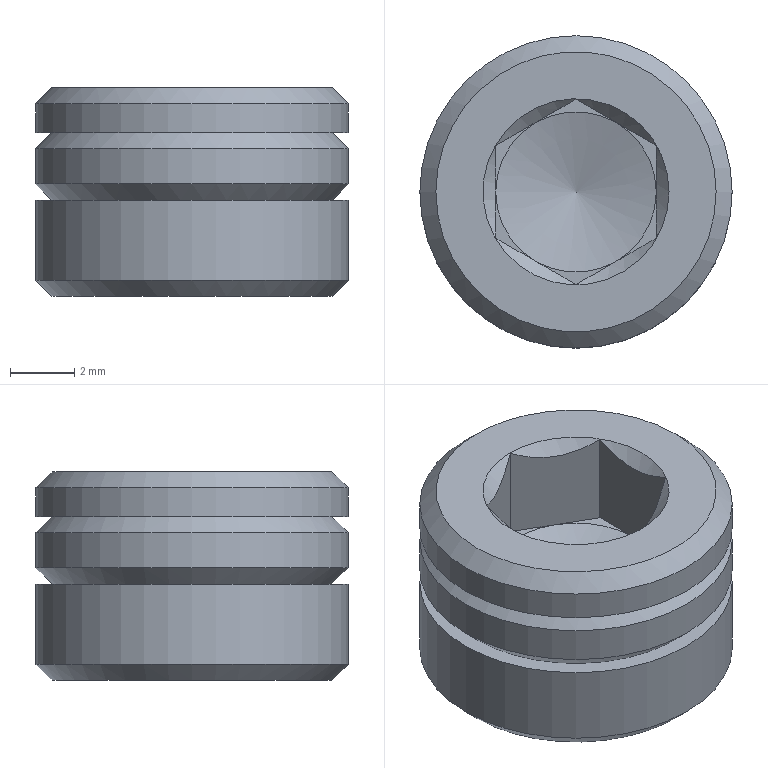Part | NX | features BREP 1 | 1 solid | 25 faces | box 9.728 x 9.728 x 6.5 mm | volume 398.103 mm3 | plane 16 | cone 6 | cylinder 3 | commonest cylinder face diameters 9.728 x3
STEP:
#1=CARTESIAN_POINT('',(4.364,0.,-6.5));
#2=VERTEX_POINT('',#1);
#3=CARTESIAN_POINT('',(0.,0.,-6.5));
#4=DIRECTION('',(0.,0.,1.));
#5=DIRECTION('',(1.,0.,0.));
#6=AXIS2_PLACEMENT_3D('',#3,#4,#5);
#7=CIRCLE('',#6,4.364);
#8=EDGE_CURVE('',#2,#2,#7,.T.);
#9=ORIENTED_EDGE('',*,*,#8,.F.);
#10=EDGE_LOOP('',(#9));
#11=FACE_BOUND('',#10,.T.);
#12=CARTESIAN_POINT('',(0.,4.364,-6.5));
#13=DIRECTION('',(0.,0.,1.));
#14=DIRECTION('',(-1.,0.,0.));
#15=AXIS2_PLACEMENT_3D('',#12,#13,#14);
#16=PLANE('',#15);
#17=ADVANCED_FACE('',(#11),#16,.F.);
#18=CARTESIAN_POINT('',(4.864,0.,-6.));
#19=VERTEX_POINT('',#18);
#20=CARTESIAN_POINT('',(0.,0.,-6.));
#21=DIRECTION('',(0.,0.,-1.));
#22=DIRECTION('',(1.,0.,0.));
#23=AXIS2_PLACEMENT_3D('',#20,#21,#22);
#24=CIRCLE('',#23,4.864);
#25=EDGE_CURVE('',#19,#19,#24,.T.);
#26=ORIENTED_EDGE('',*,*,#25,.T.);
#27=EDGE_LOOP('',(#26));
#28=FACE_BOUND('',#27,.T.);
#29=ORIENTED_EDGE('',*,*,#8,.T.);
#30=EDGE_LOOP('',(#29));
#31=FACE_BOUND('',#30,.T.);
#32=CARTESIAN_POINT('',(0.,0.,-6.));
#33=DIRECTION('',(0.,0.,1.));
#34=DIRECTION('',(-1.,0.,0.));
#35=AXIS2_PLACEMENT_3D('',#32,#33,#34);
#36=CONICAL_SURFACE('',#35,4.864,0.7854);
#37=ADVANCED_FACE('',(#28,#31),#36,.T.);
#38=CARTESIAN_POINT('',(4.864,0.,-3.5));
#39=VERTEX_POINT('',#38);
#40=CARTESIAN_POINT('',(0.,0.,-3.5));
#41=DIRECTION('',(0.,0.,-1.));
#42=DIRECTION('',(1.,0.,0.));
#43=AXIS2_PLACEMENT_3D('',#40,#41,#42);
#44=CIRCLE('',#43,4.864);
#45=EDGE_CURVE('',#39,#39,#44,.T.);
#46=ORIENTED_EDGE('',*,*,#45,.T.);
#47=EDGE_LOOP('',(#46));
#48=FACE_BOUND('',#47,.T.);
#49=ORIENTED_EDGE('',*,*,#25,.F.);
#50=EDGE_LOOP('',(#49));
#51=FACE_BOUND('',#50,.T.);
#52=CARTESIAN_POINT('',(0.,0.,-6.5));
#53=DIRECTION('',(0.,0.,1.));
#54=DIRECTION('',(-1.,0.,0.));
#55=AXIS2_PLACEMENT_3D('',#52,#53,#54);
#56=CYLINDRICAL_SURFACE('',#55,4.864);
#57=ADVANCED_FACE('',(#48,#51),#56,.T.);
#58=CARTESIAN_POINT('',(4.364,0.,-3.5));
#59=VERTEX_POINT('',#58);
#60=CARTESIAN_POINT('',(0.,0.,-3.5));
#61=DIRECTION('',(0.,0.,-1.));
#62=DIRECTION('',(1.,0.,0.));
#63=AXIS2_PLACEMENT_3D('',#60,#61,#62);
#64=CIRCLE('',#63,4.364);
#65=EDGE_CURVE('',#59,#59,#64,.T.);
#66=ORIENTED_EDGE('',*,*,#65,.T.);
#67=EDGE_LOOP('',(#66));
#68=FACE_BOUND('',#67,.T.);
#69=ORIENTED_EDGE('',*,*,#45,.F.);
#70=EDGE_LOOP('',(#69));
#71=FACE_BOUND('',#70,.T.);
#72=CARTESIAN_POINT('',(0.,4.364,-3.5));
#73=DIRECTION('',(0.,0.,1.));
#74=DIRECTION('',(-1.,0.,0.));
#75=AXIS2_PLACEMENT_3D('',#72,#73,#74);
#76=PLANE('',#75);
#77=ADVANCED_FACE('',(#68,#71),#76,.T.);
#78=ORIENTED_EDGE('',*,*,#65,.F.);
#79=EDGE_LOOP('',(#78));
#80=FACE_BOUND('',#79,.T.);
#81=CARTESIAN_POINT('',(4.864,0.,-3.));
#82=VERTEX_POINT('',#81);
#83=CARTESIAN_POINT('',(0.,0.,-3.));
#84=DIRECTION('',(0.,0.,-1.));
#85=DIRECTION('',(1.,0.,0.));
#86=AXIS2_PLACEMENT_3D('',#83,#84,#85);
#87=CIRCLE('',#86,4.864);
#88=EDGE_CURVE('',#82,#82,#87,.T.);
#89=ORIENTED_EDGE('',*,*,#88,.T.);
#90=EDGE_LOOP('',(#89));
#91=FACE_BOUND('',#90,.T.);
#92=CARTESIAN_POINT('',(0.,0.,-3.));
#93=DIRECTION('',(0.,0.,1.));
#94=DIRECTION('',(-1.,0.,0.));
#95=AXIS2_PLACEMENT_3D('',#92,#93,#94);
#96=CONICAL_SURFACE('',#95,4.864,0.7854);
#97=ADVANCED_FACE('',(#80,#91),#96,.T.);
#98=ORIENTED_EDGE('',*,*,#88,.F.);
#99=EDGE_LOOP('',(#98));
#100=FACE_BOUND('',#99,.T.);
#101=CARTESIAN_POINT('',(4.864,0.,-1.9));
#102=VERTEX_POINT('',#101);
#103=CARTESIAN_POINT('',(0.,0.,-1.9));
#104=DIRECTION('',(0.,0.,-1.));
#105=DIRECTION('',(1.,0.,0.));
#106=AXIS2_PLACEMENT_3D('',#103,#104,#105);
#107=CIRCLE('',#106,4.864);
#108=EDGE_CURVE('',#102,#102,#107,.T.);
#109=ORIENTED_EDGE('',*,*,#108,.T.);
#110=EDGE_LOOP('',(#109));
#111=FACE_BOUND('',#110,.T.);
#112=CARTESIAN_POINT('',(0.,0.,-6.5));
#113=DIRECTION('',(0.,0.,1.));
#114=DIRECTION('',(-1.,0.,0.));
#115=AXIS2_PLACEMENT_3D('',#112,#113,#114);
#116=CYLINDRICAL_SURFACE('',#115,4.864);
#117=ADVANCED_FACE('',(#100,#111),#116,.T.);
#118=CARTESIAN_POINT('',(-4.364,0.,-1.4));
#119=VERTEX_POINT('',#118);
#120=CARTESIAN_POINT('',(0.,0.,-1.4));
#121=DIRECTION('',(0.,0.,-1.));
#122=DIRECTION('',(-1.,0.,0.));
#123=AXIS2_PLACEMENT_3D('',#120,#121,#122);
#124=CIRCLE('',#123,4.364);
#125=EDGE_CURVE('',#119,#119,#124,.T.);
#126=ORIENTED_EDGE('',*,*,#125,.T.);
#127=EDGE_LOOP('',(#126));
#128=FACE_BOUND('',#127,.T.);
#129=ORIENTED_EDGE('',*,*,#108,.F.);
#130=EDGE_LOOP('',(#129));
#131=FACE_BOUND('',#130,.T.);
#132=CARTESIAN_POINT('',(0.,0.,-1.9));
#133=DIRECTION('',(0.,0.,-1.));
#134=DIRECTION('',(1.,0.,0.));
#135=AXIS2_PLACEMENT_3D('',#132,#133,#134);
#136=CONICAL_SURFACE('',#135,4.864,0.7854);
#137=ADVANCED_FACE('',(#128,#131),#136,.T.);
#138=CARTESIAN_POINT('',(4.864,0.,-1.4));
#139=VERTEX_POINT('',#138);
#140=CARTESIAN_POINT('',(0.,0.,-1.4));
#141=DIRECTION('',(0.,0.,-1.));
#142=DIRECTION('',(1.,0.,0.));
#143=AXIS2_PLACEMENT_3D('',#140,#141,#142);
#144=CIRCLE('',#143,4.864);
#145=EDGE_CURVE('',#139,#139,#144,.T.);
#146=ORIENTED_EDGE('',*,*,#145,.T.);
#147=EDGE_LOOP('',(#146));
#148=FACE_BOUND('',#147,.T.);
#149=ORIENTED_EDGE('',*,*,#125,.F.);
#150=EDGE_LOOP('',(#149));
#151=FACE_BOUND('',#150,.T.);
#152=CARTESIAN_POINT('',(0.,4.864,-1.4));
#153=DIRECTION('',(0.,0.,-1.));
#154=DIRECTION('',(1.,0.,0.));
#155=AXIS2_PLACEMENT_3D('',#152,#153,#154);
#156=PLANE('',#155);
#157=ADVANCED_FACE('',(#148,#151),#156,.T.);
#158=ORIENTED_EDGE('',*,*,#145,.F.);
#159=EDGE_LOOP('',(#158));
#160=FACE_BOUND('',#159,.T.);
#161=CARTESIAN_POINT('',(4.864,0.,-0.5));
#162=VERTEX_POINT('',#161);
#163=CARTESIAN_POINT('',(0.,0.,-0.5));
#164=DIRECTION('',(0.,0.,-1.));
#165=DIRECTION('',(1.,0.,0.));
#166=AXIS2_PLACEMENT_3D('',#163,#164,#165);
#167=CIRCLE('',#166,4.864);
#168=EDGE_CURVE('',#162,#162,#167,.T.);
#169=ORIENTED_EDGE('',*,*,#168,.T.);
#170=EDGE_LOOP('',(#169));
#171=FACE_BOUND('',#170,.T.);
#172=CARTESIAN_POINT('',(0.,0.,-6.5));
#173=DIRECTION('',(0.,0.,1.));
#174=DIRECTION('',(-1.,0.,0.));
#175=AXIS2_PLACEMENT_3D('',#172,#173,#174);
#176=CYLINDRICAL_SURFACE('',#175,4.864);
#177=ADVANCED_FACE('',(#160,#171),#176,.T.);
#178=CARTESIAN_POINT('',(-4.364,0.,0.));
#179=VERTEX_POINT('',#178);
#180=CARTESIAN_POINT('',(0.,0.,0.));
#181=DIRECTION('',(0.,0.,-1.));
#182=DIRECTION('',(-1.,0.,0.));
#183=AXIS2_PLACEMENT_3D('',#180,#181,#182);
#184=CIRCLE('',#183,4.364);
#185=EDGE_CURVE('',#179,#179,#184,.T.);
#186=ORIENTED_EDGE('',*,*,#185,.T.);
#187=EDGE_LOOP('',(#186));
#188=FACE_BOUND('',#187,.T.);
#189=ORIENTED_EDGE('',*,*,#168,.F.);
#190=EDGE_LOOP('',(#189));
#191=FACE_BOUND('',#190,.T.);
#192=CARTESIAN_POINT('',(0.,0.,-0.5));
#193=DIRECTION('',(0.,0.,-1.));
#194=DIRECTION('',(1.,0.,0.));
#195=AXIS2_PLACEMENT_3D('',#192,#193,#194);
#196=CONICAL_SURFACE('',#195,4.864,0.7854);
#197=ADVANCED_FACE('',(#188,#191),#196,.T.);
#198=ORIENTED_EDGE('',*,*,#185,.F.);
#199=EDGE_LOOP('',(#198));
#200=FACE_BOUND('',#199,.T.);
#201=CARTESIAN_POINT('',(2.9,0.,0.));
#202=VERTEX_POINT('',#201);
#203=CARTESIAN_POINT('',(0.,0.,0.));
#204=DIRECTION('',(0.,0.,1.));
#205=DIRECTION('',(1.,0.,0.));
#206=AXIS2_PLACEMENT_3D('',#203,#204,#205);
#207=CIRCLE('',#206,2.9);
#208=EDGE_CURVE('',#202,#202,#207,.T.);
#209=ORIENTED_EDGE('',*,*,#208,.F.);
#210=EDGE_LOOP('',(#209));
#211=FACE_BOUND('',#210,.T.);
#212=CARTESIAN_POINT('',(0.,0.,0.));
#213=DIRECTION('',(0.,0.,-1.));
#214=DIRECTION('',(1.,0.,0.));
#215=AXIS2_PLACEMENT_3D('',#212,#213,#214);
#216=PLANE('',#215);
#217=ADVANCED_FACE('',(#200,#211),#216,.F.);
#218=CARTESIAN_POINT('',(2.5,1.443,-0.01325));
#219=VERTEX_POINT('',#218);
#220=CARTESIAN_POINT('',(2.5,-1.443,-0.01325));
#221=VERTEX_POINT('',#220);
#222=CARTESIAN_POINT('',(2.5,1.443,-0.01325));
#223=CARTESIAN_POINT('',(2.5,0.9923,-0.2388));
#224=CARTESIAN_POINT('',(2.5,0.009298,-0.5605));
#225=CARTESIAN_POINT('',(2.5,-0.9896,-0.2401));
#226=CARTESIAN_POINT('',(2.5,-1.443,-0.01325));
#227=B_SPLINE_CURVE_WITH_KNOTS('',3,(#222,#223,#224,#225,#226),.UNSPECIFIED.,.F.,.F.,(4,1,4),(0.,0.001491,0.002982),.UNSPECIFIED.);
#228=EDGE_CURVE('',#219,#221,#227,.T.);
#229=ORIENTED_EDGE('',*,*,#228,.T.);
#230=CARTESIAN_POINT('',(-0.000000007,-2.887,-0.01325));
#231=VERTEX_POINT('',#230);
#232=CARTESIAN_POINT('',(-0.000000012,-2.887,-0.01325));
#233=CARTESIAN_POINT('',(0.3907,-2.661,-0.2388));
#234=CARTESIAN_POINT('',(1.242,-2.17,-0.5605));
#235=CARTESIAN_POINT('',(2.107,-1.67,-0.2401));
#236=CARTESIAN_POINT('',(2.5,-1.443,-0.01325));
#237=B_SPLINE_CURVE_WITH_KNOTS('',3,(#232,#233,#234,#235,#236),.UNSPECIFIED.,.F.,.F.,(4,1,4),(0.,0.001491,0.002982),.UNSPECIFIED.);
#238=EDGE_CURVE('',#231,#221,#237,.T.);
#239=ORIENTED_EDGE('',*,*,#238,.F.);
#240=CARTESIAN_POINT('',(-2.5,-1.443,-0.01325));
#241=VERTEX_POINT('',#240);
#242=CARTESIAN_POINT('',(-2.5,-1.443,-0.01325));
#243=CARTESIAN_POINT('',(-2.109,-1.669,-0.2388));
#244=CARTESIAN_POINT('',(-1.258,-2.16,-0.5605));
#245=CARTESIAN_POINT('',(-0.393,-2.66,-0.2401));
#246=CARTESIAN_POINT('',(-0.000000002,-2.887,-0.01325));
#247=B_SPLINE_CURVE_WITH_KNOTS('',3,(#242,#243,#244,#245,#246),.UNSPECIFIED.,.F.,.F.,(4,1,4),(0.,0.001491,0.002982),.UNSPECIFIED.);
#248=EDGE_CURVE('',#241,#231,#247,.T.);
#249=ORIENTED_EDGE('',*,*,#248,.F.);
#250=CARTESIAN_POINT('',(-2.5,1.443,-0.01325));
#251=VERTEX_POINT('',#250);
#252=CARTESIAN_POINT('',(-2.5,-1.443,-0.01325));
#253=CARTESIAN_POINT('',(-2.5,-0.9923,-0.2388));
#254=CARTESIAN_POINT('',(-2.5,-0.009298,-0.5605));
#255=CARTESIAN_POINT('',(-2.5,0.9896,-0.2401));
#256=CARTESIAN_POINT('',(-2.5,1.443,-0.01325));
#257=B_SPLINE_CURVE_WITH_KNOTS('',3,(#252,#253,#254,#255,#256),.UNSPECIFIED.,.F.,.F.,(4,1,4),(0.,0.001491,0.002982),.UNSPECIFIED.);
#258=EDGE_CURVE('',#241,#251,#257,.T.);
#259=ORIENTED_EDGE('',*,*,#258,.T.);
#260=CARTESIAN_POINT('',(0.000000007,2.887,-0.01325));
#261=VERTEX_POINT('',#260);
#262=CARTESIAN_POINT('',(0.000000012,2.887,-0.01325));
#263=CARTESIAN_POINT('',(-0.3907,2.661,-0.2388));
#264=CARTESIAN_POINT('',(-1.242,2.17,-0.5605));
#265=CARTESIAN_POINT('',(-2.107,1.67,-0.2401));
#266=CARTESIAN_POINT('',(-2.5,1.443,-0.01325));
#267=B_SPLINE_CURVE_WITH_KNOTS('',3,(#262,#263,#264,#265,#266),.UNSPECIFIED.,.F.,.F.,(4,1,4),(0.,0.001491,0.002982),.UNSPECIFIED.);
#268=EDGE_CURVE('',#261,#251,#267,.T.);
#269=ORIENTED_EDGE('',*,*,#268,.F.);
#270=CARTESIAN_POINT('',(2.5,1.443,-0.01325));
#271=CARTESIAN_POINT('',(2.109,1.669,-0.2388));
#272=CARTESIAN_POINT('',(1.258,2.16,-0.5605));
#273=CARTESIAN_POINT('',(0.393,2.66,-0.2401));
#274=CARTESIAN_POINT('',(0.000000002,2.887,-0.01325));
#275=B_SPLINE_CURVE_WITH_KNOTS('',3,(#270,#271,#272,#273,#274),.UNSPECIFIED.,.F.,.F.,(4,1,4),(0.,0.001491,0.002982),.UNSPECIFIED.);
#276=EDGE_CURVE('',#219,#261,#275,.T.);
#277=ORIENTED_EDGE('',*,*,#276,.F.);
#278=EDGE_LOOP('',(#229,#239,#249,#259,#269,#277));
#279=FACE_BOUND('',#278,.T.);
#280=ORIENTED_EDGE('',*,*,#208,.T.);
#281=EDGE_LOOP('',(#280));
#282=FACE_BOUND('',#281,.T.);
#283=CARTESIAN_POINT('',(0.,0.,0.));
#284=DIRECTION('',(0.,0.,1.));
#285=DIRECTION('',(-1.,0.,0.));
#286=AXIS2_PLACEMENT_3D('',#283,#284,#285);
#287=CONICAL_SURFACE('',#286,2.9,0.7854);
#288=ADVANCED_FACE('',(#279,#282),#287,.F.);
#289=CARTESIAN_POINT('',(-2.5,1.443,-3.));
#290=VERTEX_POINT('',#289);
#291=CARTESIAN_POINT('',(-2.5,1.443,-3.));
#292=DIRECTION('',(0.,0.,1.));
#293=VECTOR('',#292,1000.);
#294=LINE('',#291,#293);
#295=EDGE_CURVE('',#290,#251,#294,.T.);
#296=ORIENTED_EDGE('',*,*,#295,.F.);
#297=CARTESIAN_POINT('',(-1.25,2.165,-3.));
#298=VERTEX_POINT('',#297);
#299=CARTESIAN_POINT('',(-1.25,2.165,-3.));
#300=DIRECTION('',(-0.866,-0.5,0.));
#301=VECTOR('',#300,1000.);
#302=LINE('',#299,#301);
#303=EDGE_CURVE('',#298,#290,#302,.T.);
#304=ORIENTED_EDGE('',*,*,#303,.F.);
#305=CARTESIAN_POINT('',(0.,2.887,-3.));
#306=VERTEX_POINT('',#305);
#307=CARTESIAN_POINT('',(0.,2.887,-3.));
#308=DIRECTION('',(-0.866,-0.5,0.));
#309=VECTOR('',#308,1000.);
#310=LINE('',#307,#309);
#311=EDGE_CURVE('',#306,#298,#310,.T.);
#312=ORIENTED_EDGE('',*,*,#311,.F.);
#313=CARTESIAN_POINT('',(0.,2.887,-3.));
#314=DIRECTION('',(0.,0.,-1.));
#315=VECTOR('',#314,1000.);
#316=LINE('',#313,#315);
#317=EDGE_CURVE('',#261,#306,#316,.T.);
#318=ORIENTED_EDGE('',*,*,#317,.F.);
#319=ORIENTED_EDGE('',*,*,#268,.T.);
#320=EDGE_LOOP('',(#296,#304,#312,#318,#319));
#321=FACE_BOUND('',#320,.T.);
#322=CARTESIAN_POINT('',(0.,2.887,-3.));
#323=DIRECTION('',(-0.5,0.866,0.));
#324=DIRECTION('',(0.866,0.5,0.));
#325=AXIS2_PLACEMENT_3D('',#322,#323,#324);
#326=PLANE('',#325);
#327=ADVANCED_FACE('',(#321),#326,.F.);
#328=ORIENTED_EDGE('',*,*,#317,.T.);
#329=CARTESIAN_POINT('',(1.25,2.165,-3.));
#330=VERTEX_POINT('',#329);
#331=CARTESIAN_POINT('',(1.25,2.165,-3.));
#332=DIRECTION('',(-0.866,0.5,0.));
#333=VECTOR('',#332,1000.);
#334=LINE('',#331,#333);
#335=EDGE_CURVE('',#330,#306,#334,.T.);
#336=ORIENTED_EDGE('',*,*,#335,.F.);
#337=CARTESIAN_POINT('',(2.5,1.443,-3.));
#338=VERTEX_POINT('',#337);
#339=CARTESIAN_POINT('',(2.5,1.443,-3.));
#340=DIRECTION('',(-0.866,0.5,0.));
#341=VECTOR('',#340,1000.);
#342=LINE('',#339,#341);
#343=EDGE_CURVE('',#338,#330,#342,.T.);
#344=ORIENTED_EDGE('',*,*,#343,.F.);
#345=CARTESIAN_POINT('',(2.5,1.443,-3.));
#346=DIRECTION('',(0.,0.,-1.));
#347=VECTOR('',#346,1000.);
#348=LINE('',#345,#347);
#349=EDGE_CURVE('',#219,#338,#348,.T.);
#350=ORIENTED_EDGE('',*,*,#349,.F.);
#351=ORIENTED_EDGE('',*,*,#276,.T.);
#352=EDGE_LOOP('',(#328,#336,#344,#350,#351));
#353=FACE_BOUND('',#352,.T.);
#354=CARTESIAN_POINT('',(2.5,1.443,-3.));
#355=DIRECTION('',(0.5,0.866,0.));
#356=DIRECTION('',(0.866,-0.5,0.));
#357=AXIS2_PLACEMENT_3D('',#354,#355,#356);
#358=PLANE('',#357);
#359=ADVANCED_FACE('',(#353),#358,.F.);
#360=CARTESIAN_POINT('',(2.5,-1.443,-3.));
#361=VERTEX_POINT('',#360);
#362=CARTESIAN_POINT('',(2.5,-1.443,-3.));
#363=DIRECTION('',(0.,0.,1.));
#364=VECTOR('',#363,1000.);
#365=LINE('',#362,#364);
#366=EDGE_CURVE('',#361,#221,#365,.T.);
#367=ORIENTED_EDGE('',*,*,#366,.F.);
#368=CARTESIAN_POINT('',(1.25,-2.165,-3.));
#369=VERTEX_POINT('',#368);
#370=CARTESIAN_POINT('',(1.25,-2.165,-3.));
#371=DIRECTION('',(0.866,0.5,0.));
#372=VECTOR('',#371,1000.);
#373=LINE('',#370,#372);
#374=EDGE_CURVE('',#369,#361,#373,.T.);
#375=ORIENTED_EDGE('',*,*,#374,.F.);
#376=CARTESIAN_POINT('',(0.,-2.887,-3.));
#377=VERTEX_POINT('',#376);
#378=CARTESIAN_POINT('',(0.,-2.887,-3.));
#379=DIRECTION('',(0.866,0.5,0.));
#380=VECTOR('',#379,1000.);
#381=LINE('',#378,#380);
#382=EDGE_CURVE('',#377,#369,#381,.T.);
#383=ORIENTED_EDGE('',*,*,#382,.F.);
#384=CARTESIAN_POINT('',(0.,-2.887,-3.));
#385=DIRECTION('',(0.,0.,-1.));
#386=VECTOR('',#385,1000.);
#387=LINE('',#384,#386);
#388=EDGE_CURVE('',#231,#377,#387,.T.);
#389=ORIENTED_EDGE('',*,*,#388,.F.);
#390=ORIENTED_EDGE('',*,*,#238,.T.);
#391=EDGE_LOOP('',(#367,#375,#383,#389,#390));
#392=FACE_BOUND('',#391,.T.);
#393=CARTESIAN_POINT('',(0.,-2.887,-3.));
#394=DIRECTION('',(0.5,-0.866,0.));
#395=DIRECTION('',(-0.866,-0.5,0.));
#396=AXIS2_PLACEMENT_3D('',#393,#394,#395);
#397=PLANE('',#396);
#398=ADVANCED_FACE('',(#392),#397,.F.);
#399=ORIENTED_EDGE('',*,*,#388,.T.);
#400=CARTESIAN_POINT('',(-1.25,-2.165,-3.));
#401=VERTEX_POINT('',#400);
#402=CARTESIAN_POINT('',(-1.25,-2.165,-3.));
#403=DIRECTION('',(0.866,-0.5,0.));
#404=VECTOR('',#403,1000.);
#405=LINE('',#402,#404);
#406=EDGE_CURVE('',#401,#377,#405,.T.);
#407=ORIENTED_EDGE('',*,*,#406,.F.);
#408=CARTESIAN_POINT('',(-2.5,-1.443,-3.));
#409=VERTEX_POINT('',#408);
#410=CARTESIAN_POINT('',(-2.5,-1.443,-3.));
#411=DIRECTION('',(0.866,-0.5,0.));
#412=VECTOR('',#411,1000.);
#413=LINE('',#410,#412);
#414=EDGE_CURVE('',#409,#401,#413,.T.);
#415=ORIENTED_EDGE('',*,*,#414,.F.);
#416=CARTESIAN_POINT('',(-2.5,-1.443,-3.));
#417=DIRECTION('',(0.,0.,-1.));
#418=VECTOR('',#417,1000.);
#419=LINE('',#416,#418);
#420=EDGE_CURVE('',#241,#409,#419,.T.);
#421=ORIENTED_EDGE('',*,*,#420,.F.);
#422=ORIENTED_EDGE('',*,*,#248,.T.);
#423=EDGE_LOOP('',(#399,#407,#415,#421,#422));
#424=FACE_BOUND('',#423,.T.);
#425=CARTESIAN_POINT('',(-2.5,-1.443,-3.));
#426=DIRECTION('',(-0.5,-0.866,0.));
#427=DIRECTION('',(-0.866,0.5,0.));
#428=AXIS2_PLACEMENT_3D('',#425,#426,#427);
#429=PLANE('',#428);
#430=ADVANCED_FACE('',(#424),#429,.F.);
#431=ORIENTED_EDGE('',*,*,#420,.T.);
#432=CARTESIAN_POINT('',(-2.5,0.,-3.));
#433=VERTEX_POINT('',#432);
#434=CARTESIAN_POINT('',(-2.5,1.443,-3.));
#435=DIRECTION('',(0.,-1.,0.));
#436=VECTOR('',#435,1000.);
#437=LINE('',#434,#436);
#438=EDGE_CURVE('',#433,#409,#437,.T.);
#439=ORIENTED_EDGE('',*,*,#438,.F.);
#440=CARTESIAN_POINT('',(-2.5,0.,-3.));
#441=DIRECTION('',(0.,-1.,0.));
#442=VECTOR('',#441,1000.);
#443=LINE('',#440,#442);
#444=EDGE_CURVE('',#290,#433,#443,.T.);
#445=ORIENTED_EDGE('',*,*,#444,.F.);
#446=ORIENTED_EDGE('',*,*,#295,.T.);
#447=ORIENTED_EDGE('',*,*,#258,.F.);
#448=EDGE_LOOP('',(#431,#439,#445,#446,#447));
#449=FACE_BOUND('',#448,.T.);
#450=CARTESIAN_POINT('',(-2.5,1.443,-3.));
#451=DIRECTION('',(-1.,0.,0.));
#452=DIRECTION('',(0.,0.,-1.));
#453=AXIS2_PLACEMENT_3D('',#450,#451,#452);
#454=PLANE('',#453);
#455=ADVANCED_FACE('',(#449),#454,.F.);
#456=ORIENTED_EDGE('',*,*,#349,.T.);
#457=CARTESIAN_POINT('',(2.5,0.,-3.));
#458=VERTEX_POINT('',#457);
#459=CARTESIAN_POINT('',(2.5,0.,-3.));
#460=DIRECTION('',(0.,1.,0.));
#461=VECTOR('',#460,1000.);
#462=LINE('',#459,#461);
#463=EDGE_CURVE('',#458,#338,#462,.T.);
#464=ORIENTED_EDGE('',*,*,#463,.F.);
#465=CARTESIAN_POINT('',(2.5,0.,-3.));
#466=DIRECTION('',(0.,1.,0.));
#467=VECTOR('',#466,1000.);
#468=LINE('',#465,#467);
#469=EDGE_CURVE('',#361,#458,#468,.T.);
#470=ORIENTED_EDGE('',*,*,#469,.F.);
#471=ORIENTED_EDGE('',*,*,#366,.T.);
#472=ORIENTED_EDGE('',*,*,#228,.F.);
#473=EDGE_LOOP('',(#456,#464,#470,#471,#472));
#474=FACE_BOUND('',#473,.T.);
#475=CARTESIAN_POINT('',(2.5,-1.443,-3.));
#476=DIRECTION('',(1.,0.,0.));
#477=DIRECTION('',(0.,0.,1.));
#478=AXIS2_PLACEMENT_3D('',#475,#476,#477);
#479=PLANE('',#478);
#480=ADVANCED_FACE('',(#474),#479,.F.);
#481=ORIENTED_EDGE('',*,*,#438,.T.);
#482=ORIENTED_EDGE('',*,*,#414,.T.);
#483=CARTESIAN_POINT('',(0.,0.,-3.));
#484=DIRECTION('',(0.,0.,-1.));
#485=DIRECTION('',(1.,0.,0.));
#486=AXIS2_PLACEMENT_3D('',#483,#484,#485);
#487=CIRCLE('',#486,2.5);
#488=EDGE_CURVE('',#401,#433,#487,.T.);
#489=ORIENTED_EDGE('',*,*,#488,.T.);
#490=EDGE_LOOP('',(#481,#482,#489));
#491=FACE_BOUND('',#490,.T.);
#492=CARTESIAN_POINT('',(0.,0.,-3.));
#493=DIRECTION('',(0.,0.,1.));
#494=DIRECTION('',(-1.,0.,0.));
#495=AXIS2_PLACEMENT_3D('',#492,#493,#494);
#496=PLANE('',#495);
#497=ADVANCED_FACE('',(#491),#496,.T.);
#498=CARTESIAN_POINT('',(0.,0.,-3.693));
#499=VERTEX_POINT('',#498);
#500=VERTEX_LOOP('',#499);
#501=FACE_BOUND('',#500,.T.);
#502=CARTESIAN_POINT('',(0.,0.,-3.));
#503=DIRECTION('',(0.,0.,-1.));
#504=DIRECTION('',(1.,0.,0.));
#505=AXIS2_PLACEMENT_3D('',#502,#503,#504);
#506=CIRCLE('',#505,2.5);
#507=EDGE_CURVE('',#433,#298,#506,.T.);
#508=ORIENTED_EDGE('',*,*,#507,.F.);
#509=ORIENTED_EDGE('',*,*,#488,.F.);
#510=CARTESIAN_POINT('',(0.,0.,-3.));
#511=DIRECTION('',(0.,0.,-1.));
#512=DIRECTION('',(1.,0.,0.));
#513=AXIS2_PLACEMENT_3D('',#510,#511,#512);
#514=CIRCLE('',#513,2.5);
#515=EDGE_CURVE('',#369,#401,#514,.T.);
#516=ORIENTED_EDGE('',*,*,#515,.F.);
#517=CARTESIAN_POINT('',(0.,0.,-3.));
#518=DIRECTION('',(0.,0.,-1.));
#519=DIRECTION('',(1.,0.,0.));
#520=AXIS2_PLACEMENT_3D('',#517,#518,#519);
#521=CIRCLE('',#520,2.5);
#522=EDGE_CURVE('',#458,#369,#521,.T.);
#523=ORIENTED_EDGE('',*,*,#522,.F.);
#524=CARTESIAN_POINT('',(0.,0.,-3.));
#525=DIRECTION('',(0.,0.,-1.));
#526=DIRECTION('',(1.,0.,0.));
#527=AXIS2_PLACEMENT_3D('',#524,#525,#526);
#528=CIRCLE('',#527,2.5);
#529=EDGE_CURVE('',#330,#458,#528,.T.);
#530=ORIENTED_EDGE('',*,*,#529,.F.);
#531=CARTESIAN_POINT('',(0.,0.,-3.));
#532=DIRECTION('',(0.,0.,-1.));
#533=DIRECTION('',(1.,0.,0.));
#534=AXIS2_PLACEMENT_3D('',#531,#532,#533);
#535=CIRCLE('',#534,2.5);
#536=EDGE_CURVE('',#298,#330,#535,.T.);
#537=ORIENTED_EDGE('',*,*,#536,.F.);
#538=EDGE_LOOP('',(#508,#509,#516,#523,#530,#537));
#539=FACE_BOUND('',#538,.T.);
#540=CARTESIAN_POINT('',(0.,0.,-3.));
#541=DIRECTION('',(0.,0.,1.));
#542=DIRECTION('',(-1.,0.,0.));
#543=AXIS2_PLACEMENT_3D('',#540,#541,#542);
#544=CONICAL_SURFACE('',#543,2.5,1.3);
#545=ADVANCED_FACE('',(#501,#539),#544,.F.);
#546=ORIENTED_EDGE('',*,*,#406,.T.);
#547=ORIENTED_EDGE('',*,*,#382,.T.);
#548=ORIENTED_EDGE('',*,*,#515,.T.);
#549=EDGE_LOOP('',(#546,#547,#548));
#550=FACE_BOUND('',#549,.T.);
#551=CARTESIAN_POINT('',(0.,0.,-3.));
#552=DIRECTION('',(0.,0.,1.));
#553=DIRECTION('',(-1.,0.,0.));
#554=AXIS2_PLACEMENT_3D('',#551,#552,#553);
#555=PLANE('',#554);
#556=ADVANCED_FACE('',(#550),#555,.T.);
#557=ORIENTED_EDGE('',*,*,#374,.T.);
#558=ORIENTED_EDGE('',*,*,#469,.T.);
#559=ORIENTED_EDGE('',*,*,#522,.T.);
#560=EDGE_LOOP('',(#557,#558,#559));
#561=FACE_BOUND('',#560,.T.);
#562=CARTESIAN_POINT('',(0.,0.,-3.));
#563=DIRECTION('',(0.,0.,1.));
#564=DIRECTION('',(-1.,0.,0.));
#565=AXIS2_PLACEMENT_3D('',#562,#563,#564);
#566=PLANE('',#565);
#567=ADVANCED_FACE('',(#561),#566,.T.);
#568=ORIENTED_EDGE('',*,*,#463,.T.);
#569=ORIENTED_EDGE('',*,*,#343,.T.);
#570=ORIENTED_EDGE('',*,*,#529,.T.);
#571=EDGE_LOOP('',(#568,#569,#570));
#572=FACE_BOUND('',#571,.T.);
#573=CARTESIAN_POINT('',(0.,0.,-3.));
#574=DIRECTION('',(0.,0.,1.));
#575=DIRECTION('',(-1.,0.,0.));
#576=AXIS2_PLACEMENT_3D('',#573,#574,#575);
#577=PLANE('',#576);
#578=ADVANCED_FACE('',(#572),#577,.T.);
#579=ORIENTED_EDGE('',*,*,#335,.T.);
#580=ORIENTED_EDGE('',*,*,#311,.T.);
#581=ORIENTED_EDGE('',*,*,#536,.T.);
#582=EDGE_LOOP('',(#579,#580,#581));
#583=FACE_BOUND('',#582,.T.);
#584=CARTESIAN_POINT('',(0.,0.,-3.));
#585=DIRECTION('',(0.,0.,1.));
#586=DIRECTION('',(-1.,0.,0.));
#587=AXIS2_PLACEMENT_3D('',#584,#585,#586);
#588=PLANE('',#587);
#589=ADVANCED_FACE('',(#583),#588,.T.);
#590=ORIENTED_EDGE('',*,*,#303,.T.);
#591=ORIENTED_EDGE('',*,*,#444,.T.);
#592=ORIENTED_EDGE('',*,*,#507,.T.);
#593=EDGE_LOOP('',(#590,#591,#592));
#594=FACE_BOUND('',#593,.T.);
#595=CARTESIAN_POINT('',(0.,0.,-3.));
#596=DIRECTION('',(0.,0.,1.));
#597=DIRECTION('',(-1.,0.,0.));
#598=AXIS2_PLACEMENT_3D('',#595,#596,#597);
#599=PLANE('',#598);
#600=ADVANCED_FACE('',(#594),#599,.T.);
#601=CLOSED_SHELL('',(#17,#37,#57,#77,#97,#117,#137,#157,#177,#197,#217,#288,#327,#359,#398,#430,#455,#480,#497,#545,#556,#567,#578,#589,#600));
#602=MANIFOLD_SOLID_BREP('',#601);
#603=(LENGTH_UNIT()NAMED_UNIT(*)SI_UNIT(.MILLI.,.METRE.));
#604=UNCERTAINTY_MEASURE_WITH_UNIT(LENGTH_MEASURE(0.0508),#603,'','');
#605=(NAMED_UNIT(*)PLANE_ANGLE_UNIT()SI_UNIT($,.RADIAN.));
#606=(NAMED_UNIT(*)SI_UNIT($,.STERADIAN.)SOLID_ANGLE_UNIT());
#607=(GEOMETRIC_REPRESENTATION_CONTEXT(3)GLOBAL_UNCERTAINTY_ASSIGNED_CONTEXT((#604))GLOBAL_UNIT_ASSIGNED_CONTEXT((#603,#605,#606))REPRESENTATION_CONTEXT('',''));
#608=ADVANCED_BREP_SHAPE_REPRESENTATION('',(#602),#607);